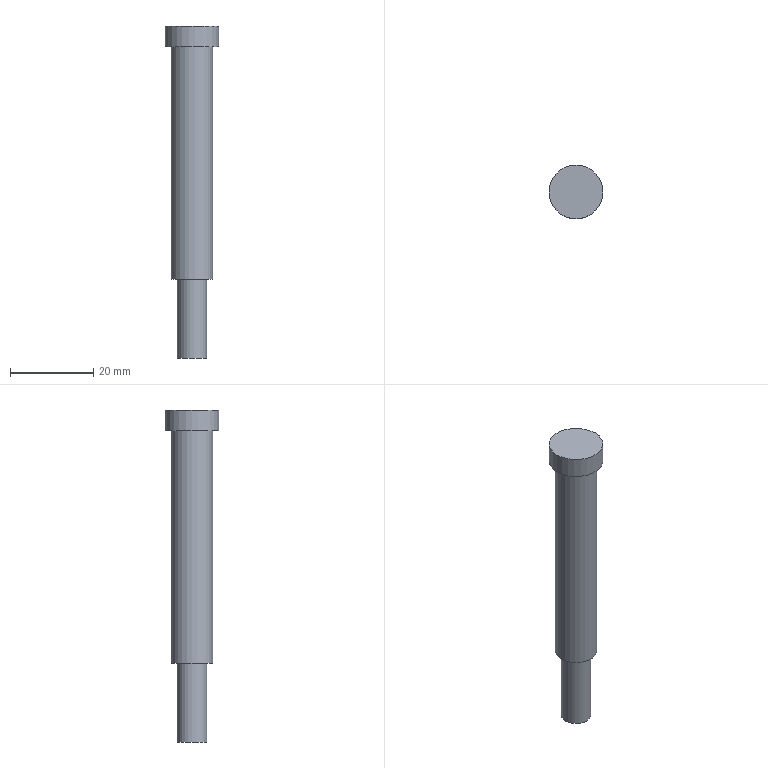Part | NX | features solid 2 | 1 solid | 7 faces | box 13 x 13 x 80 mm | volume 5814 mm3 | plane 4 | cylinder 3 | commonest cylinder face diameters 7.1 x1 10 x1 13 x1
STEP:
#1=CARTESIAN_POINT('',(-251.705,234.513,48.));
#2=VERTEX_POINT('',#1);
#3=CARTESIAN_POINT('',(-256.705,234.513,48.));
#4=DIRECTION('',(0.,0.,1.));
#5=DIRECTION('',(1.,0.,0.));
#6=AXIS2_PLACEMENT_3D('',#3,#4,#5);
#7=CIRCLE('',#6,5.);
#8=EDGE_CURVE('',#2,#2,#7,.T.);
#9=ORIENTED_EDGE('',*,*,#8,.T.);
#10=EDGE_LOOP('',(#9));
#11=FACE_BOUND('',#10,.T.);
#12=CARTESIAN_POINT('',(-251.705,234.513,104.));
#13=VERTEX_POINT('',#12);
#14=CARTESIAN_POINT('',(-256.705,234.513,104.));
#15=DIRECTION('',(0.,0.,1.));
#16=DIRECTION('',(1.,0.,0.));
#17=AXIS2_PLACEMENT_3D('',#14,#15,#16);
#18=CIRCLE('',#17,5.);
#19=EDGE_CURVE('',#13,#13,#18,.T.);
#20=ORIENTED_EDGE('',*,*,#19,.F.);
#21=EDGE_LOOP('',(#20));
#22=FACE_BOUND('',#21,.T.);
#23=CARTESIAN_POINT('',(-256.705,234.513,109.));
#24=DIRECTION('',(0.,0.,-1.));
#25=DIRECTION('',(-1.,0.,0.));
#26=AXIS2_PLACEMENT_3D('',#23,#24,#25);
#27=CYLINDRICAL_SURFACE('',#26,5.);
#28=ADVANCED_FACE('',(#11,#22),#27,.T.);
#29=CARTESIAN_POINT('',(-253.155,234.513,48.));
#30=VERTEX_POINT('',#29);
#31=CARTESIAN_POINT('',(-256.705,234.513,48.));
#32=DIRECTION('',(0.,0.,1.));
#33=DIRECTION('',(1.,0.,0.));
#34=AXIS2_PLACEMENT_3D('',#31,#32,#33);
#35=CIRCLE('',#34,3.55);
#36=EDGE_CURVE('',#30,#30,#35,.T.);
#37=ORIENTED_EDGE('',*,*,#36,.T.);
#38=EDGE_LOOP('',(#37));
#39=FACE_BOUND('',#38,.T.);
#40=ORIENTED_EDGE('',*,*,#8,.F.);
#41=EDGE_LOOP('',(#40));
#42=FACE_BOUND('',#41,.T.);
#43=CARTESIAN_POINT('',(-256.705,234.513,48.));
#44=DIRECTION('',(0.,0.,1.));
#45=DIRECTION('',(1.,0.,0.));
#46=AXIS2_PLACEMENT_3D('',#43,#44,#45);
#47=PLANE('',#46);
#48=ADVANCED_FACE('',(#39,#42),#47,.F.);
#49=CARTESIAN_POINT('',(-250.205,234.513,104.));
#50=VERTEX_POINT('',#49);
#51=CARTESIAN_POINT('',(-256.705,234.513,104.));
#52=DIRECTION('',(0.,0.,1.));
#53=DIRECTION('',(1.,0.,0.));
#54=AXIS2_PLACEMENT_3D('',#51,#52,#53);
#55=CIRCLE('',#54,6.5);
#56=EDGE_CURVE('',#50,#50,#55,.T.);
#57=ORIENTED_EDGE('',*,*,#56,.F.);
#58=EDGE_LOOP('',(#57));
#59=FACE_BOUND('',#58,.T.);
#60=ORIENTED_EDGE('',*,*,#19,.T.);
#61=EDGE_LOOP('',(#60));
#62=FACE_BOUND('',#61,.T.);
#63=CARTESIAN_POINT('',(-256.705,234.513,104.));
#64=DIRECTION('',(0.,0.,1.));
#65=DIRECTION('',(1.,0.,0.));
#66=AXIS2_PLACEMENT_3D('',#63,#64,#65);
#67=PLANE('',#66);
#68=ADVANCED_FACE('',(#59,#62),#67,.F.);
#69=ORIENTED_EDGE('',*,*,#56,.T.);
#70=EDGE_LOOP('',(#69));
#71=FACE_BOUND('',#70,.T.);
#72=CARTESIAN_POINT('',(-250.205,234.513,109.));
#73=VERTEX_POINT('',#72);
#74=CARTESIAN_POINT('',(-256.705,234.513,109.));
#75=DIRECTION('',(0.,0.,1.));
#76=DIRECTION('',(1.,0.,0.));
#77=AXIS2_PLACEMENT_3D('',#74,#75,#76);
#78=CIRCLE('',#77,6.5);
#79=EDGE_CURVE('',#73,#73,#78,.T.);
#80=ORIENTED_EDGE('',*,*,#79,.F.);
#81=EDGE_LOOP('',(#80));
#82=FACE_BOUND('',#81,.T.);
#83=CARTESIAN_POINT('',(-256.705,234.513,104.));
#84=DIRECTION('',(0.,0.,1.));
#85=DIRECTION('',(1.,0.,0.));
#86=AXIS2_PLACEMENT_3D('',#83,#84,#85);
#87=CYLINDRICAL_SURFACE('',#86,6.5);
#88=ADVANCED_FACE('',(#71,#82),#87,.T.);
#89=ORIENTED_EDGE('',*,*,#79,.T.);
#90=EDGE_LOOP('',(#89));
#91=FACE_BOUND('',#90,.T.);
#92=CARTESIAN_POINT('',(-256.705,234.513,109.));
#93=DIRECTION('',(0.,0.,1.));
#94=DIRECTION('',(1.,0.,0.));
#95=AXIS2_PLACEMENT_3D('',#92,#93,#94);
#96=PLANE('',#95);
#97=ADVANCED_FACE('',(#91),#96,.T.);
#98=CARTESIAN_POINT('',(-253.155,234.513,29.));
#99=VERTEX_POINT('',#98);
#100=CARTESIAN_POINT('',(-256.705,234.513,29.));
#101=DIRECTION('',(0.,0.,1.));
#102=DIRECTION('',(1.,0.,0.));
#103=AXIS2_PLACEMENT_3D('',#100,#101,#102);
#104=CIRCLE('',#103,3.55);
#105=EDGE_CURVE('',#99,#99,#104,.T.);
#106=ORIENTED_EDGE('',*,*,#105,.T.);
#107=EDGE_LOOP('',(#106));
#108=FACE_BOUND('',#107,.T.);
#109=ORIENTED_EDGE('',*,*,#36,.F.);
#110=EDGE_LOOP('',(#109));
#111=FACE_BOUND('',#110,.T.);
#112=CARTESIAN_POINT('',(-256.705,234.513,29.));
#113=DIRECTION('',(0.,0.,1.));
#114=DIRECTION('',(1.,0.,0.));
#115=AXIS2_PLACEMENT_3D('',#112,#113,#114);
#116=CYLINDRICAL_SURFACE('',#115,3.55);
#117=ADVANCED_FACE('',(#108,#111),#116,.T.);
#118=ORIENTED_EDGE('',*,*,#105,.F.);
#119=EDGE_LOOP('',(#118));
#120=FACE_BOUND('',#119,.T.);
#121=CARTESIAN_POINT('',(-256.705,234.513,29.));
#122=DIRECTION('',(0.,0.,1.));
#123=DIRECTION('',(1.,0.,0.));
#124=AXIS2_PLACEMENT_3D('',#121,#122,#123);
#125=PLANE('',#124);
#126=ADVANCED_FACE('',(#120),#125,.F.);
#127=CLOSED_SHELL('',(#28,#48,#68,#88,#97,#117,#126));
#128=MANIFOLD_SOLID_BREP('',#127);
#129=(LENGTH_UNIT()NAMED_UNIT(*)SI_UNIT(.MILLI.,.METRE.));
#130=UNCERTAINTY_MEASURE_WITH_UNIT(LENGTH_MEASURE(0.00001),#129,'','');
#131=(NAMED_UNIT(*)PLANE_ANGLE_UNIT()SI_UNIT($,.RADIAN.));
#132=(NAMED_UNIT(*)SI_UNIT($,.STERADIAN.)SOLID_ANGLE_UNIT());
#133=(GEOMETRIC_REPRESENTATION_CONTEXT(3)GLOBAL_UNCERTAINTY_ASSIGNED_CONTEXT((#130))GLOBAL_UNIT_ASSIGNED_CONTEXT((#129,#131,#132))REPRESENTATION_CONTEXT('',''));
#134=ADVANCED_BREP_SHAPE_REPRESENTATION('',(#128),#133);